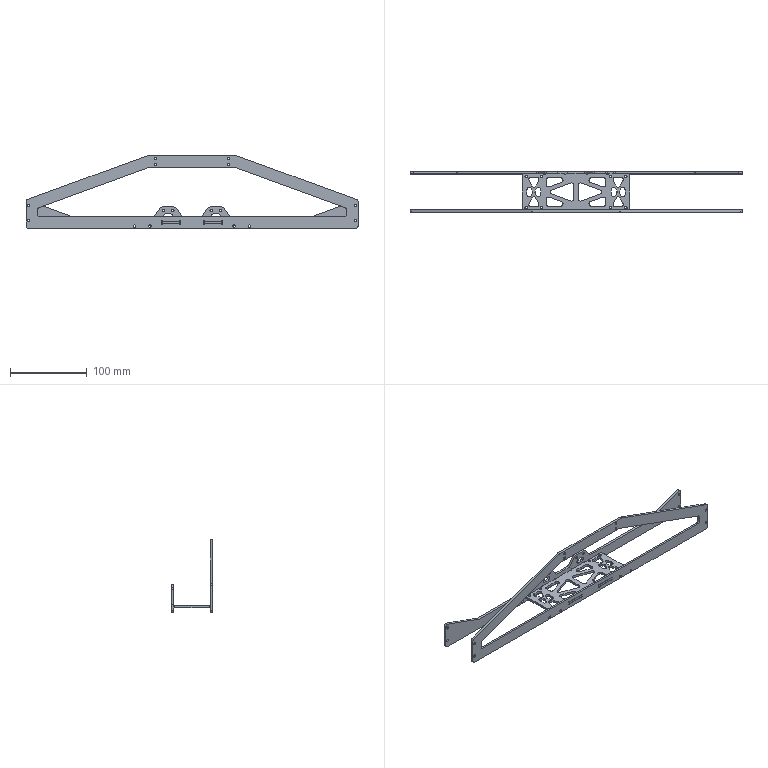Part | SolidWorks | features Fillet 6, ICE 4, Extrusion 1 | 3 solids | 329 faces | box 433.1 x 53 x 95 mm | volume 77453 mm3 | cylinder 215 | plane 114 | commonest cylinder face diameters 6 x87 3.2 x64 1.5 x28 2 x20 1 x16